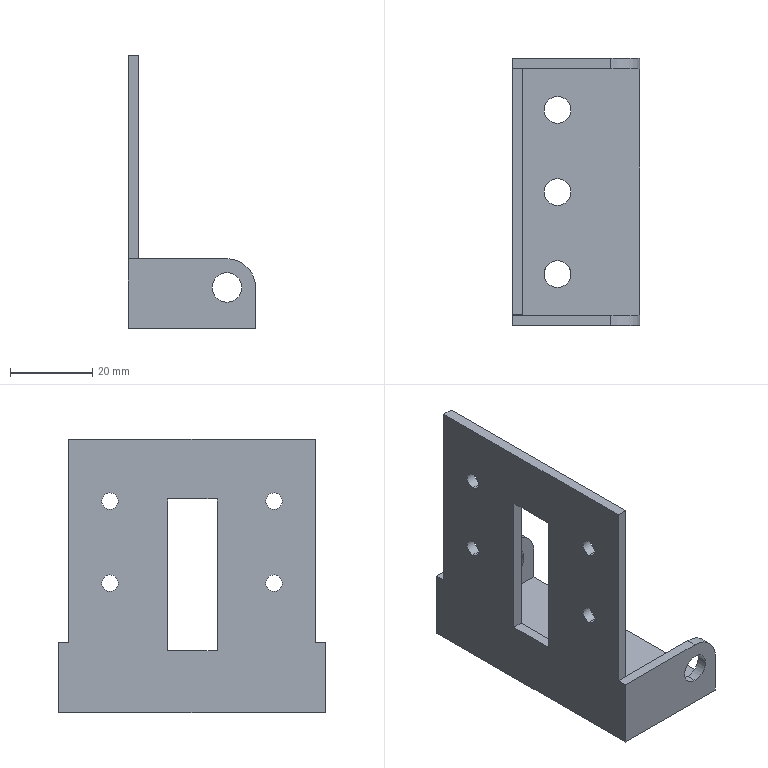Part | SolidWorks | features BaseBody 1 | 1 solid | 38 faces | box 31 x 65 x 66.5 mm | volume 15144 mm3 | cylinder 20 | plane 18 | commonest cylinder face diameters 4 x8 6.5 x6 7.2 x4 14 x2
STEP:
#1=CARTESIAN_POINT('',(875.446,-3880.873,994.471));
#2=VERTEX_POINT('',#1);
#3=CARTESIAN_POINT('',(875.446,-3880.873,998.471));
#4=VERTEX_POINT('',#3);
#5=CARTESIAN_POINT('',(875.446,-3880.873,996.471));
#6=DIRECTION('',(-1.,0.,0.));
#7=DIRECTION('',(0.,0.,1.));
#8=AXIS2_PLACEMENT_3D('',#5,#6,#7);
#9=CIRCLE('',#8,2.);
#10=EDGE_CURVE('',#2,#4,#9,.T.);
#11=ORIENTED_EDGE('',*,*,#10,.F.);
#12=CARTESIAN_POINT('',(872.946,-3880.873,994.471));
#13=VERTEX_POINT('',#12);
#14=CARTESIAN_POINT('',(787.194,-3880.873,994.471));
#15=DIRECTION('',(-1.,0.,0.));
#16=VECTOR('',#15,1000.);
#17=LINE('',#14,#16);
#18=EDGE_CURVE('',#2,#13,#17,.T.);
#19=ORIENTED_EDGE('',*,*,#18,.T.);
#20=CARTESIAN_POINT('',(872.946,-3880.873,998.471));
#21=VERTEX_POINT('',#20);
#22=CARTESIAN_POINT('',(872.946,-3880.873,996.471));
#23=DIRECTION('',(1.,0.,0.));
#24=DIRECTION('',(0.,0.,1.));
#25=AXIS2_PLACEMENT_3D('',#22,#23,#24);
#26=CIRCLE('',#25,2.);
#27=EDGE_CURVE('',#21,#13,#26,.T.);
#28=ORIENTED_EDGE('',*,*,#27,.F.);
#29=CARTESIAN_POINT('',(787.194,-3880.873,998.471));
#30=DIRECTION('',(-1.,0.,0.));
#31=VECTOR('',#30,1000.);
#32=LINE('',#29,#31);
#33=EDGE_CURVE('',#4,#21,#32,.T.);
#34=ORIENTED_EDGE('',*,*,#33,.F.);
#35=EDGE_LOOP('',(#11,#19,#28,#34));
#36=FACE_OUTER_BOUND('',#35,.T.);
#37=CARTESIAN_POINT('',(787.194,-3880.873,996.471));
#38=DIRECTION('',(-1.,0.,0.));
#39=DIRECTION('',(0.,0.,1.));
#40=AXIS2_PLACEMENT_3D('',#37,#38,#39);
#41=CYLINDRICAL_SURFACE('',#40,2.);
#42=ADVANCED_FACE('',(#36),#41,.F.);
#43=CARTESIAN_POINT('',(875.446,-3880.873,974.471));
#44=VERTEX_POINT('',#43);
#45=CARTESIAN_POINT('',(875.446,-3880.873,978.471));
#46=VERTEX_POINT('',#45);
#47=CARTESIAN_POINT('',(875.446,-3880.873,976.471));
#48=DIRECTION('',(-1.,0.,0.));
#49=DIRECTION('',(0.,0.,1.));
#50=AXIS2_PLACEMENT_3D('',#47,#48,#49);
#51=CIRCLE('',#50,2.);
#52=EDGE_CURVE('',#44,#46,#51,.T.);
#53=ORIENTED_EDGE('',*,*,#52,.F.);
#54=CARTESIAN_POINT('',(872.946,-3880.873,974.471));
#55=VERTEX_POINT('',#54);
#56=CARTESIAN_POINT('',(787.194,-3880.873,974.471));
#57=DIRECTION('',(-1.,0.,0.));
#58=VECTOR('',#57,1000.);
#59=LINE('',#56,#58);
#60=EDGE_CURVE('',#44,#55,#59,.T.);
#61=ORIENTED_EDGE('',*,*,#60,.T.);
#62=CARTESIAN_POINT('',(872.946,-3880.873,978.471));
#63=VERTEX_POINT('',#62);
#64=CARTESIAN_POINT('',(872.946,-3880.873,976.471));
#65=DIRECTION('',(1.,0.,0.));
#66=DIRECTION('',(0.,0.,1.));
#67=AXIS2_PLACEMENT_3D('',#64,#65,#66);
#68=CIRCLE('',#67,2.);
#69=EDGE_CURVE('',#63,#55,#68,.T.);
#70=ORIENTED_EDGE('',*,*,#69,.F.);
#71=CARTESIAN_POINT('',(787.194,-3880.873,978.471));
#72=DIRECTION('',(-1.,0.,0.));
#73=VECTOR('',#72,1000.);
#74=LINE('',#71,#73);
#75=EDGE_CURVE('',#46,#63,#74,.T.);
#76=ORIENTED_EDGE('',*,*,#75,.F.);
#77=EDGE_LOOP('',(#53,#61,#70,#76));
#78=FACE_OUTER_BOUND('',#77,.T.);
#79=CARTESIAN_POINT('',(787.194,-3880.873,976.471));
#80=DIRECTION('',(-1.,0.,0.));
#81=DIRECTION('',(0.,0.,1.));
#82=AXIS2_PLACEMENT_3D('',#79,#80,#81);
#83=CYLINDRICAL_SURFACE('',#82,2.);
#84=ADVANCED_FACE('',(#78),#83,.F.);
#85=CARTESIAN_POINT('',(872.946,-3920.873,978.471));
#86=VERTEX_POINT('',#85);
#87=CARTESIAN_POINT('',(872.946,-3920.873,974.471));
#88=VERTEX_POINT('',#87);
#89=CARTESIAN_POINT('',(872.946,-3920.873,976.471));
#90=DIRECTION('',(1.,0.,0.));
#91=DIRECTION('',(0.,0.,-1.));
#92=AXIS2_PLACEMENT_3D('',#89,#90,#91);
#93=CIRCLE('',#92,2.);
#94=EDGE_CURVE('',#86,#88,#93,.T.);
#95=ORIENTED_EDGE('',*,*,#94,.F.);
#96=CARTESIAN_POINT('',(875.446,-3920.873,978.471));
#97=VERTEX_POINT('',#96);
#98=CARTESIAN_POINT('',(787.194,-3920.873,978.471));
#99=DIRECTION('',(1.,0.,0.));
#100=VECTOR('',#99,1000.);
#101=LINE('',#98,#100);
#102=EDGE_CURVE('',#86,#97,#101,.T.);
#103=ORIENTED_EDGE('',*,*,#102,.T.);
#104=CARTESIAN_POINT('',(875.446,-3920.873,974.471));
#105=VERTEX_POINT('',#104);
#106=CARTESIAN_POINT('',(875.446,-3920.873,976.471));
#107=DIRECTION('',(-1.,0.,0.));
#108=DIRECTION('',(0.,0.,-1.));
#109=AXIS2_PLACEMENT_3D('',#106,#107,#108);
#110=CIRCLE('',#109,2.);
#111=EDGE_CURVE('',#105,#97,#110,.T.);
#112=ORIENTED_EDGE('',*,*,#111,.F.);
#113=CARTESIAN_POINT('',(787.194,-3920.873,974.471));
#114=DIRECTION('',(1.,0.,0.));
#115=VECTOR('',#114,1000.);
#116=LINE('',#113,#115);
#117=EDGE_CURVE('',#88,#105,#116,.T.);
#118=ORIENTED_EDGE('',*,*,#117,.F.);
#119=EDGE_LOOP('',(#95,#103,#112,#118));
#120=FACE_OUTER_BOUND('',#119,.T.);
#121=CARTESIAN_POINT('',(787.194,-3920.873,976.471));
#122=DIRECTION('',(1.,0.,0.));
#123=DIRECTION('',(0.,0.,-1.));
#124=AXIS2_PLACEMENT_3D('',#121,#122,#123);
#125=CYLINDRICAL_SURFACE('',#124,2.);
#126=ADVANCED_FACE('',(#120),#125,.F.);
#127=CARTESIAN_POINT('',(872.946,-3920.873,998.471));
#128=VERTEX_POINT('',#127);
#129=CARTESIAN_POINT('',(872.946,-3920.873,994.471));
#130=VERTEX_POINT('',#129);
#131=CARTESIAN_POINT('',(872.946,-3920.873,996.471));
#132=DIRECTION('',(1.,0.,0.));
#133=DIRECTION('',(0.,0.,-1.));
#134=AXIS2_PLACEMENT_3D('',#131,#132,#133);
#135=CIRCLE('',#134,2.);
#136=EDGE_CURVE('',#128,#130,#135,.T.);
#137=ORIENTED_EDGE('',*,*,#136,.F.);
#138=CARTESIAN_POINT('',(875.446,-3920.873,998.471));
#139=VERTEX_POINT('',#138);
#140=CARTESIAN_POINT('',(787.194,-3920.873,998.471));
#141=DIRECTION('',(1.,0.,0.));
#142=VECTOR('',#141,1000.);
#143=LINE('',#140,#142);
#144=EDGE_CURVE('',#128,#139,#143,.T.);
#145=ORIENTED_EDGE('',*,*,#144,.T.);
#146=CARTESIAN_POINT('',(875.446,-3920.873,994.471));
#147=VERTEX_POINT('',#146);
#148=CARTESIAN_POINT('',(875.446,-3920.873,996.471));
#149=DIRECTION('',(-1.,0.,0.));
#150=DIRECTION('',(0.,0.,-1.));
#151=AXIS2_PLACEMENT_3D('',#148,#149,#150);
#152=CIRCLE('',#151,2.);
#153=EDGE_CURVE('',#147,#139,#152,.T.);
#154=ORIENTED_EDGE('',*,*,#153,.F.);
#155=CARTESIAN_POINT('',(787.194,-3920.873,994.471));
#156=DIRECTION('',(1.,0.,0.));
#157=VECTOR('',#156,1000.);
#158=LINE('',#155,#157);
#159=EDGE_CURVE('',#130,#147,#158,.T.);
#160=ORIENTED_EDGE('',*,*,#159,.F.);
#161=EDGE_LOOP('',(#137,#145,#154,#160));
#162=FACE_OUTER_BOUND('',#161,.T.);
#163=CARTESIAN_POINT('',(787.194,-3920.873,996.471));
#164=DIRECTION('',(1.,0.,0.));
#165=DIRECTION('',(0.,0.,-1.));
#166=AXIS2_PLACEMENT_3D('',#163,#164,#165);
#167=CYLINDRICAL_SURFACE('',#166,2.);
#168=ADVANCED_FACE('',(#162),#167,.F.);
#169=CARTESIAN_POINT('',(896.946,-3930.873,958.571));
#170=VERTEX_POINT('',#169);
#171=CARTESIAN_POINT('',(896.946,-3930.873,951.371));
#172=VERTEX_POINT('',#171);
#173=CARTESIAN_POINT('',(896.946,-3930.873,954.971));
#174=DIRECTION('',(0.,-1.,0.));
#175=DIRECTION('',(0.,0.,-1.));
#176=AXIS2_PLACEMENT_3D('',#173,#174,#175);
#177=CIRCLE('',#176,3.6);
#178=EDGE_CURVE('',#170,#172,#177,.T.);
#179=ORIENTED_EDGE('',*,*,#178,.F.);
#180=CARTESIAN_POINT('',(896.946,-3933.373,958.571));
#181=VERTEX_POINT('',#180);
#182=CARTESIAN_POINT('',(896.946,-3930.873,958.571));
#183=DIRECTION('',(0.,-1.,0.));
#184=VECTOR('',#183,1000.);
#185=LINE('',#182,#184);
#186=EDGE_CURVE('',#170,#181,#185,.T.);
#187=ORIENTED_EDGE('',*,*,#186,.T.);
#188=CARTESIAN_POINT('',(896.946,-3933.373,951.371));
#189=VERTEX_POINT('',#188);
#190=CARTESIAN_POINT('',(896.946,-3933.373,954.971));
#191=DIRECTION('',(0.,-1.,0.));
#192=DIRECTION('',(0.,0.,-1.));
#193=AXIS2_PLACEMENT_3D('',#190,#191,#192);
#194=CIRCLE('',#193,3.6);
#195=EDGE_CURVE('',#181,#189,#194,.T.);
#196=ORIENTED_EDGE('',*,*,#195,.T.);
#197=CARTESIAN_POINT('',(896.946,-3930.873,951.371));
#198=DIRECTION('',(0.,-1.,0.));
#199=VECTOR('',#198,1000.);
#200=LINE('',#197,#199);
#201=EDGE_CURVE('',#172,#189,#200,.T.);
#202=ORIENTED_EDGE('',*,*,#201,.F.);
#203=EDGE_LOOP('',(#179,#187,#196,#202));
#204=FACE_OUTER_BOUND('',#203,.T.);
#205=CARTESIAN_POINT('',(896.946,-3930.873,954.971));
#206=DIRECTION('',(0.,-1.,0.));
#207=DIRECTION('',(0.,0.,-1.));
#208=AXIS2_PLACEMENT_3D('',#205,#206,#207);
#209=CYLINDRICAL_SURFACE('',#208,3.6);
#210=ADVANCED_FACE('',(#204),#209,.F.);
#211=CARTESIAN_POINT('',(880.696,-3900.873,944.971));
#212=VERTEX_POINT('',#211);
#213=CARTESIAN_POINT('',(887.196,-3900.873,944.971));
#214=VERTEX_POINT('',#213);
#215=CARTESIAN_POINT('',(883.946,-3900.873,944.971));
#216=DIRECTION('',(0.,0.,1.));
#217=DIRECTION('',(1.,0.,0.));
#218=AXIS2_PLACEMENT_3D('',#215,#216,#217);
#219=CIRCLE('',#218,3.25);
#220=EDGE_CURVE('',#212,#214,#219,.T.);
#221=ORIENTED_EDGE('',*,*,#220,.F.);
#222=CARTESIAN_POINT('',(880.696,-3900.873,947.471));
#223=VERTEX_POINT('',#222);
#224=CARTESIAN_POINT('',(880.696,-3900.873,970.533));
#225=DIRECTION('',(0.,0.,1.));
#226=VECTOR('',#225,1000.);
#227=LINE('',#224,#226);
#228=EDGE_CURVE('',#212,#223,#227,.T.);
#229=ORIENTED_EDGE('',*,*,#228,.T.);
#230=CARTESIAN_POINT('',(887.196,-3900.873,947.471));
#231=VERTEX_POINT('',#230);
#232=CARTESIAN_POINT('',(883.946,-3900.873,947.471));
#233=DIRECTION('',(0.,0.,-1.));
#234=DIRECTION('',(1.,0.,0.));
#235=AXIS2_PLACEMENT_3D('',#232,#233,#234);
#236=CIRCLE('',#235,3.25);
#237=EDGE_CURVE('',#231,#223,#236,.T.);
#238=ORIENTED_EDGE('',*,*,#237,.F.);
#239=CARTESIAN_POINT('',(887.196,-3900.873,970.533));
#240=DIRECTION('',(0.,0.,1.));
#241=VECTOR('',#240,1000.);
#242=LINE('',#239,#241);
#243=EDGE_CURVE('',#214,#231,#242,.T.);
#244=ORIENTED_EDGE('',*,*,#243,.F.);
#245=EDGE_LOOP('',(#221,#229,#238,#244));
#246=FACE_OUTER_BOUND('',#245,.T.);
#247=CARTESIAN_POINT('',(883.946,-3900.873,970.533));
#248=DIRECTION('',(0.,0.,1.));
#249=DIRECTION('',(1.,0.,0.));
#250=AXIS2_PLACEMENT_3D('',#247,#248,#249);
#251=CYLINDRICAL_SURFACE('',#250,3.25);
#252=ADVANCED_FACE('',(#246),#251,.F.);
#253=CARTESIAN_POINT('',(880.696,-3880.873,944.971));
#254=VERTEX_POINT('',#253);
#255=CARTESIAN_POINT('',(887.196,-3880.873,944.971));
#256=VERTEX_POINT('',#255);
#257=CARTESIAN_POINT('',(883.946,-3880.873,944.971));
#258=DIRECTION('',(0.,0.,1.));
#259=DIRECTION('',(1.,0.,0.));
#260=AXIS2_PLACEMENT_3D('',#257,#258,#259);
#261=CIRCLE('',#260,3.25);
#262=EDGE_CURVE('',#254,#256,#261,.T.);
#263=ORIENTED_EDGE('',*,*,#262,.F.);
#264=CARTESIAN_POINT('',(880.696,-3880.873,947.471));
#265=VERTEX_POINT('',#264);
#266=CARTESIAN_POINT('',(880.696,-3880.873,970.533));
#267=DIRECTION('',(0.,0.,1.));
#268=VECTOR('',#267,1000.);
#269=LINE('',#266,#268);
#270=EDGE_CURVE('',#254,#265,#269,.T.);
#271=ORIENTED_EDGE('',*,*,#270,.T.);
#272=CARTESIAN_POINT('',(887.196,-3880.873,947.471));
#273=VERTEX_POINT('',#272);
#274=CARTESIAN_POINT('',(883.946,-3880.873,947.471));
#275=DIRECTION('',(0.,0.,-1.));
#276=DIRECTION('',(1.,0.,0.));
#277=AXIS2_PLACEMENT_3D('',#274,#275,#276);
#278=CIRCLE('',#277,3.25);
#279=EDGE_CURVE('',#273,#265,#278,.T.);
#280=ORIENTED_EDGE('',*,*,#279,.F.);
#281=CARTESIAN_POINT('',(887.196,-3880.873,970.533));
#282=DIRECTION('',(0.,0.,1.));
#283=VECTOR('',#282,1000.);
#284=LINE('',#281,#283);
#285=EDGE_CURVE('',#256,#273,#284,.T.);
#286=ORIENTED_EDGE('',*,*,#285,.F.);
#287=EDGE_LOOP('',(#263,#271,#280,#286));
#288=FACE_OUTER_BOUND('',#287,.T.);
#289=CARTESIAN_POINT('',(883.946,-3880.873,970.533));
#290=DIRECTION('',(0.,0.,1.));
#291=DIRECTION('',(1.,0.,0.));
#292=AXIS2_PLACEMENT_3D('',#289,#290,#291);
#293=CYLINDRICAL_SURFACE('',#292,3.25);
#294=ADVANCED_FACE('',(#288),#293,.F.);
#295=CARTESIAN_POINT('',(880.696,-3920.873,944.971));
#296=VERTEX_POINT('',#295);
#297=CARTESIAN_POINT('',(887.196,-3920.873,944.971));
#298=VERTEX_POINT('',#297);
#299=CARTESIAN_POINT('',(883.946,-3920.873,944.971));
#300=DIRECTION('',(0.,0.,1.));
#301=DIRECTION('',(1.,0.,0.));
#302=AXIS2_PLACEMENT_3D('',#299,#300,#301);
#303=CIRCLE('',#302,3.25);
#304=EDGE_CURVE('',#296,#298,#303,.T.);
#305=ORIENTED_EDGE('',*,*,#304,.F.);
#306=CARTESIAN_POINT('',(880.696,-3920.873,947.471));
#307=VERTEX_POINT('',#306);
#308=CARTESIAN_POINT('',(880.696,-3920.873,970.533));
#309=DIRECTION('',(0.,0.,1.));
#310=VECTOR('',#309,1000.);
#311=LINE('',#308,#310);
#312=EDGE_CURVE('',#296,#307,#311,.T.);
#313=ORIENTED_EDGE('',*,*,#312,.T.);
#314=CARTESIAN_POINT('',(887.196,-3920.873,947.471));
#315=VERTEX_POINT('',#314);
#316=CARTESIAN_POINT('',(883.946,-3920.873,947.471));
#317=DIRECTION('',(0.,0.,-1.));
#318=DIRECTION('',(1.,0.,0.));
#319=AXIS2_PLACEMENT_3D('',#316,#317,#318);
#320=CIRCLE('',#319,3.25);
#321=EDGE_CURVE('',#315,#307,#320,.T.);
#322=ORIENTED_EDGE('',*,*,#321,.F.);
#323=CARTESIAN_POINT('',(887.196,-3920.873,970.533));
#324=DIRECTION('',(0.,0.,1.));
#325=VECTOR('',#324,1000.);
#326=LINE('',#323,#325);
#327=EDGE_CURVE('',#298,#315,#326,.T.);
#328=ORIENTED_EDGE('',*,*,#327,.F.);
#329=EDGE_LOOP('',(#305,#313,#322,#328));
#330=FACE_OUTER_BOUND('',#329,.T.);
#331=CARTESIAN_POINT('',(883.946,-3920.873,970.533));
#332=DIRECTION('',(0.,0.,1.));
#333=DIRECTION('',(1.,0.,0.));
#334=AXIS2_PLACEMENT_3D('',#331,#332,#333);
#335=CYLINDRICAL_SURFACE('',#334,3.25);
#336=ADVANCED_FACE('',(#330),#335,.F.);
#337=CARTESIAN_POINT('',(896.946,-3868.373,951.371));
#338=VERTEX_POINT('',#337);
#339=CARTESIAN_POINT('',(896.946,-3868.373,958.571));
#340=VERTEX_POINT('',#339);
#341=CARTESIAN_POINT('',(896.946,-3868.373,954.971));
#342=DIRECTION('',(0.,1.,0.));
#343=DIRECTION('',(0.,0.,-1.));
#344=AXIS2_PLACEMENT_3D('',#341,#342,#343);
#345=CIRCLE('',#344,3.6);
#346=EDGE_CURVE('',#338,#340,#345,.T.);
#347=ORIENTED_EDGE('',*,*,#346,.T.);
#348=CARTESIAN_POINT('',(896.946,-3870.873,958.571));
#349=VERTEX_POINT('',#348);
#350=CARTESIAN_POINT('',(896.946,-3868.373,958.571));
#351=DIRECTION('',(0.,-1.,0.));
#352=VECTOR('',#351,1000.);
#353=LINE('',#350,#352);
#354=EDGE_CURVE('',#340,#349,#353,.T.);
#355=ORIENTED_EDGE('',*,*,#354,.T.);
#356=CARTESIAN_POINT('',(896.946,-3870.873,951.371));
#357=VERTEX_POINT('',#356);
#358=CARTESIAN_POINT('',(896.946,-3870.873,954.971));
#359=DIRECTION('',(0.,1.,0.));
#360=DIRECTION('',(0.,0.,-1.));
#361=AXIS2_PLACEMENT_3D('',#358,#359,#360);
#362=CIRCLE('',#361,3.6);
#363=EDGE_CURVE('',#357,#349,#362,.T.);
#364=ORIENTED_EDGE('',*,*,#363,.F.);
#365=CARTESIAN_POINT('',(896.946,-3868.373,951.371));
#366=DIRECTION('',(0.,-1.,0.));
#367=VECTOR('',#366,1000.);
#368=LINE('',#365,#367);
#369=EDGE_CURVE('',#338,#357,#368,.T.);
#370=ORIENTED_EDGE('',*,*,#369,.F.);
#371=EDGE_LOOP('',(#347,#355,#364,#370));
#372=FACE_OUTER_BOUND('',#371,.T.);
#373=CARTESIAN_POINT('',(896.946,-3868.373,954.971));
#374=DIRECTION('',(0.,-1.,0.));
#375=DIRECTION('',(0.,0.,-1.));
#376=AXIS2_PLACEMENT_3D('',#373,#374,#375);
#377=CYLINDRICAL_SURFACE('',#376,3.6);
#378=ADVANCED_FACE('',(#372),#377,.F.);
#379=CARTESIAN_POINT('',(872.946,-3870.873,1011.471));
#380=VERTEX_POINT('',#379);
#381=CARTESIAN_POINT('',(872.946,-3870.873,961.971));
#382=VERTEX_POINT('',#381);
#383=CARTESIAN_POINT('',(872.946,-3870.873,951.471));
#384=DIRECTION('',(0.,0.,-1.));
#385=VECTOR('',#384,1000.);
#386=LINE('',#383,#385);
#387=EDGE_CURVE('',#380,#382,#386,.T.);
#388=ORIENTED_EDGE('',*,*,#387,.T.);
#389=CARTESIAN_POINT('',(872.946,-3868.373,961.971));
#390=VERTEX_POINT('',#389);
#391=CARTESIAN_POINT('',(872.946,-3870.873,961.971));
#392=DIRECTION('',(0.,1.,0.));
#393=VECTOR('',#392,1000.);
#394=LINE('',#391,#393);
#395=EDGE_CURVE('',#382,#390,#394,.T.);
#396=ORIENTED_EDGE('',*,*,#395,.T.);
#397=CARTESIAN_POINT('',(872.946,-3868.373,944.971));
#398=VERTEX_POINT('',#397);
#399=CARTESIAN_POINT('',(872.946,-3868.373,951.471));
#400=DIRECTION('',(0.,0.,-1.));
#401=VECTOR('',#400,1000.);
#402=LINE('',#399,#401);
#403=EDGE_CURVE('',#390,#398,#402,.T.);
#404=ORIENTED_EDGE('',*,*,#403,.T.);
#405=CARTESIAN_POINT('',(872.946,-3933.373,944.971));
#406=VERTEX_POINT('',#405);
#407=CARTESIAN_POINT('',(872.946,-3870.873,944.971));
#408=DIRECTION('',(0.,-1.,0.));
#409=VECTOR('',#408,1000.);
#410=LINE('',#407,#409);
#411=EDGE_CURVE('',#398,#406,#410,.T.);
#412=ORIENTED_EDGE('',*,*,#411,.T.);
#413=CARTESIAN_POINT('',(872.946,-3933.373,961.971));
#414=VERTEX_POINT('',#413);
#415=CARTESIAN_POINT('',(872.946,-3933.373,951.471));
#416=DIRECTION('',(0.,0.,1.));
#417=VECTOR('',#416,1000.);
#418=LINE('',#415,#417);
#419=EDGE_CURVE('',#406,#414,#418,.T.);
#420=ORIENTED_EDGE('',*,*,#419,.T.);
#421=CARTESIAN_POINT('',(872.946,-3930.873,961.971));
#422=VERTEX_POINT('',#421);
#423=CARTESIAN_POINT('',(872.946,-3870.873,961.971));
#424=DIRECTION('',(0.,1.,0.));
#425=VECTOR('',#424,1000.);
#426=LINE('',#423,#425);
#427=EDGE_CURVE('',#414,#422,#426,.T.);
#428=ORIENTED_EDGE('',*,*,#427,.T.);
#429=CARTESIAN_POINT('',(872.946,-3930.873,1011.471));
#430=VERTEX_POINT('',#429);
#431=CARTESIAN_POINT('',(872.946,-3930.873,951.471));
#432=DIRECTION('',(0.,0.,1.));
#433=VECTOR('',#432,1000.);
#434=LINE('',#431,#433);
#435=EDGE_CURVE('',#422,#430,#434,.T.);
#436=ORIENTED_EDGE('',*,*,#435,.T.);
#437=CARTESIAN_POINT('',(872.946,-3870.873,1011.471));
#438=DIRECTION('',(0.,1.,0.));
#439=VECTOR('',#438,1000.);
#440=LINE('',#437,#439);
#441=EDGE_CURVE('',#430,#380,#440,.T.);
#442=ORIENTED_EDGE('',*,*,#441,.T.);
#443=EDGE_LOOP('',(#388,#396,#404,#412,#420,#428,#436,#442));
#444=FACE_OUTER_BOUND('',#443,.T.);
#445=CARTESIAN_POINT('',(872.946,-3894.973,959.971));
#446=VERTEX_POINT('',#445);
#447=CARTESIAN_POINT('',(872.946,-3894.973,996.971));
#448=VERTEX_POINT('',#447);
#449=CARTESIAN_POINT('',(872.946,-3894.973,951.471));
#450=DIRECTION('',(0.,0.,1.));
#451=VECTOR('',#450,1000.);
#452=LINE('',#449,#451);
#453=EDGE_CURVE('',#446,#448,#452,.T.);
#454=ORIENTED_EDGE('',*,*,#453,.T.);
#455=CARTESIAN_POINT('',(872.946,-3906.973,996.971));
#456=VERTEX_POINT('',#455);
#457=CARTESIAN_POINT('',(872.946,-3870.873,996.971));
#458=DIRECTION('',(0.,-1.,0.));
#459=VECTOR('',#458,1000.);
#460=LINE('',#457,#459);
#461=EDGE_CURVE('',#448,#456,#460,.T.);
#462=ORIENTED_EDGE('',*,*,#461,.T.);
#463=CARTESIAN_POINT('',(872.946,-3906.973,959.971));
#464=VERTEX_POINT('',#463);
#465=CARTESIAN_POINT('',(872.946,-3906.973,951.471));
#466=DIRECTION('',(0.,0.,-1.));
#467=VECTOR('',#466,1000.);
#468=LINE('',#465,#467);
#469=EDGE_CURVE('',#456,#464,#468,.T.);
#470=ORIENTED_EDGE('',*,*,#469,.T.);
#471=CARTESIAN_POINT('',(872.946,-3870.873,959.971));
#472=DIRECTION('',(0.,1.,0.));
#473=VECTOR('',#472,1000.);
#474=LINE('',#471,#473);
#475=EDGE_CURVE('',#464,#446,#474,.T.);
#476=ORIENTED_EDGE('',*,*,#475,.T.);
#477=EDGE_LOOP('',(#454,#462,#470,#476));
#478=FACE_BOUND('',#477,.T.);
#479=ORIENTED_EDGE('',*,*,#27,.T.);
#480=CARTESIAN_POINT('',(872.946,-3880.873,996.471));
#481=DIRECTION('',(1.,0.,0.));
#482=DIRECTION('',(0.,0.,1.));
#483=AXIS2_PLACEMENT_3D('',#480,#481,#482);
#484=CIRCLE('',#483,2.);
#485=EDGE_CURVE('',#13,#21,#484,.T.);
#486=ORIENTED_EDGE('',*,*,#485,.T.);
#487=EDGE_LOOP('',(#479,#486));
#488=FACE_BOUND('',#487,.T.);
#489=ORIENTED_EDGE('',*,*,#69,.T.);
#490=CARTESIAN_POINT('',(872.946,-3880.873,976.471));
#491=DIRECTION('',(1.,0.,0.));
#492=DIRECTION('',(0.,0.,1.));
#493=AXIS2_PLACEMENT_3D('',#490,#491,#492);
#494=CIRCLE('',#493,2.);
#495=EDGE_CURVE('',#55,#63,#494,.T.);
#496=ORIENTED_EDGE('',*,*,#495,.T.);
#497=EDGE_LOOP('',(#489,#496));
#498=FACE_BOUND('',#497,.T.);
#499=CARTESIAN_POINT('',(872.946,-3920.873,976.471));
#500=DIRECTION('',(1.,0.,0.));
#501=DIRECTION('',(0.,0.,-1.));
#502=AXIS2_PLACEMENT_3D('',#499,#500,#501);
#503=CIRCLE('',#502,2.);
#504=EDGE_CURVE('',#88,#86,#503,.T.);
#505=ORIENTED_EDGE('',*,*,#504,.T.);
#506=ORIENTED_EDGE('',*,*,#94,.T.);
#507=EDGE_LOOP('',(#505,#506));
#508=FACE_BOUND('',#507,.T.);
#509=CARTESIAN_POINT('',(872.946,-3920.873,996.471));
#510=DIRECTION('',(1.,0.,0.));
#511=DIRECTION('',(0.,0.,-1.));
#512=AXIS2_PLACEMENT_3D('',#509,#510,#511);
#513=CIRCLE('',#512,2.);
#514=EDGE_CURVE('',#130,#128,#513,.T.);
#515=ORIENTED_EDGE('',*,*,#514,.T.);
#516=ORIENTED_EDGE('',*,*,#136,.T.);
#517=EDGE_LOOP('',(#515,#516));
#518=FACE_BOUND('',#517,.T.);
#519=CARTESIAN_POINT('',(872.946,-3870.873,951.471));
#520=DIRECTION('',(-1.,0.,0.));
#521=DIRECTION('',(0.,0.,1.));
#522=AXIS2_PLACEMENT_3D('',#519,#520,#521);
#523=PLANE('',#522);
#524=ADVANCED_FACE('',(#444,#478,#488,#498,#508,#518),#523,.T.);
#525=CARTESIAN_POINT('',(875.446,-3870.873,961.971));
#526=VERTEX_POINT('',#525);
#527=CARTESIAN_POINT('',(896.946,-3870.873,961.971));
#528=VERTEX_POINT('',#527);
#529=CARTESIAN_POINT('',(872.946,-3870.873,961.971));
#530=DIRECTION('',(1.,0.,0.));
#531=VECTOR('',#530,1000.);
#532=LINE('',#529,#531);
#533=EDGE_CURVE('',#526,#528,#532,.T.);
#534=ORIENTED_EDGE('',*,*,#533,.T.);
#535=CARTESIAN_POINT('',(896.946,-3868.373,961.971));
#536=VERTEX_POINT('',#535);
#537=CARTESIAN_POINT('',(896.946,-3870.873,961.971));
#538=DIRECTION('',(0.,1.,0.));
#539=VECTOR('',#538,1000.);
#540=LINE('',#537,#539);
#541=EDGE_CURVE('',#528,#536,#540,.T.);
#542=ORIENTED_EDGE('',*,*,#541,.T.);
#543=CARTESIAN_POINT('',(872.946,-3868.373,961.971));
#544=DIRECTION('',(-1.,0.,0.));
#545=VECTOR('',#544,1000.);
#546=LINE('',#543,#545);
#547=EDGE_CURVE('',#536,#390,#546,.T.);
#548=ORIENTED_EDGE('',*,*,#547,.T.);
#549=ORIENTED_EDGE('',*,*,#395,.F.);
#550=CARTESIAN_POINT('',(872.946,-3870.873,961.971));
#551=DIRECTION('',(1.,0.,0.));
#552=VECTOR('',#551,1000.);
#553=LINE('',#550,#552);
#554=EDGE_CURVE('',#382,#526,#553,.T.);
#555=ORIENTED_EDGE('',*,*,#554,.T.);
#556=EDGE_LOOP('',(#534,#542,#548,#549,#555));
#557=FACE_OUTER_BOUND('',#556,.T.);
#558=CARTESIAN_POINT('',(872.946,-3870.873,961.971));
#559=DIRECTION('',(0.,0.,1.));
#560=DIRECTION('',(1.,0.,0.));
#561=AXIS2_PLACEMENT_3D('',#558,#559,#560);
#562=PLANE('',#561);
#563=ADVANCED_FACE('',(#557),#562,.T.);
#564=CARTESIAN_POINT('',(875.446,-3870.873,1011.471));
#565=VERTEX_POINT('',#564);
#566=CARTESIAN_POINT('',(879.441,-3870.873,1011.471));
#567=DIRECTION('',(1.,0.,0.));
#568=VECTOR('',#567,1000.);
#569=LINE('',#566,#568);
#570=EDGE_CURVE('',#380,#565,#569,.T.);
#571=ORIENTED_EDGE('',*,*,#570,.T.);
#572=CARTESIAN_POINT('',(875.446,-3870.873,965.967));
#573=DIRECTION('',(0.,0.,-1.));
#574=VECTOR('',#573,1000.);
#575=LINE('',#572,#574);
#576=EDGE_CURVE('',#565,#526,#575,.T.);
#577=ORIENTED_EDGE('',*,*,#576,.T.);
#578=ORIENTED_EDGE('',*,*,#554,.F.);
#579=ORIENTED_EDGE('',*,*,#387,.F.);
#580=EDGE_LOOP('',(#571,#577,#578,#579));
#581=FACE_OUTER_BOUND('',#580,.T.);
#582=CARTESIAN_POINT('',(879.441,-3870.873,965.967));
#583=DIRECTION('',(0.,1.,0.));
#584=DIRECTION('',(0.,0.,1.));
#585=AXIS2_PLACEMENT_3D('',#582,#583,#584);
#586=PLANE('',#585);
#587=ADVANCED_FACE('',(#581),#586,.T.);
#588=ORIENTED_EDGE('',*,*,#570,.F.);
#589=ORIENTED_EDGE('',*,*,#441,.F.);
#590=CARTESIAN_POINT('',(875.446,-3930.873,1011.471));
#591=VERTEX_POINT('',#590);
#592=CARTESIAN_POINT('',(872.946,-3930.873,1011.471));
#593=DIRECTION('',(1.,0.,0.));
#594=VECTOR('',#593,1000.);
#595=LINE('',#592,#594);
#596=EDGE_CURVE('',#430,#591,#595,.T.);
#597=ORIENTED_EDGE('',*,*,#596,.T.);
#598=CARTESIAN_POINT('',(875.446,-3870.873,1011.471));
#599=DIRECTION('',(0.,1.,0.));
#600=VECTOR('',#599,1000.);
#601=LINE('',#598,#600);
#602=EDGE_CURVE('',#591,#565,#601,.T.);
#603=ORIENTED_EDGE('',*,*,#602,.T.);
#604=EDGE_LOOP('',(#588,#589,#597,#603));
#605=FACE_OUTER_BOUND('',#604,.T.);
#606=CARTESIAN_POINT('',(872.946,-3870.873,1011.471));
#607=DIRECTION('',(0.,0.,1.));
#608=DIRECTION('',(1.,0.,0.));
#609=AXIS2_PLACEMENT_3D('',#606,#607,#608);
#610=PLANE('',#609);
#611=ADVANCED_FACE('',(#605),#610,.T.);
#612=CARTESIAN_POINT('',(875.446,-3930.873,961.971));
#613=VERTEX_POINT('',#612);
#614=CARTESIAN_POINT('',(875.446,-3930.873,965.967));
#615=DIRECTION('',(0.,0.,-1.));
#616=VECTOR('',#615,1000.);
#617=LINE('',#614,#616);
#618=EDGE_CURVE('',#591,#613,#617,.T.);
#619=ORIENTED_EDGE('',*,*,#618,.F.);
#620=ORIENTED_EDGE('',*,*,#596,.F.);
#621=ORIENTED_EDGE('',*,*,#435,.F.);
#622=CARTESIAN_POINT('',(879.441,-3930.873,961.971));
#623=DIRECTION('',(-1.,0.,0.));
#624=VECTOR('',#623,1000.);
#625=LINE('',#622,#624);
#626=EDGE_CURVE('',#613,#422,#625,.T.);
#627=ORIENTED_EDGE('',*,*,#626,.F.);
#628=EDGE_LOOP('',(#619,#620,#621,#627));
#629=FACE_OUTER_BOUND('',#628,.T.);
#630=CARTESIAN_POINT('',(879.441,-3930.873,965.967));
#631=DIRECTION('',(0.,1.,0.));
#632=DIRECTION('',(0.,0.,1.));
#633=AXIS2_PLACEMENT_3D('',#630,#631,#632);
#634=PLANE('',#633);
#635=ADVANCED_FACE('',(#629),#634,.F.);
#636=ORIENTED_EDGE('',*,*,#626,.T.);
#637=ORIENTED_EDGE('',*,*,#427,.F.);
#638=CARTESIAN_POINT('',(896.946,-3933.373,961.971));
#639=VERTEX_POINT('',#638);
#640=CARTESIAN_POINT('',(872.946,-3933.373,961.971));
#641=DIRECTION('',(1.,0.,0.));
#642=VECTOR('',#641,1000.);
#643=LINE('',#640,#642);
#644=EDGE_CURVE('',#414,#639,#643,.T.);
#645=ORIENTED_EDGE('',*,*,#644,.T.);
#646=CARTESIAN_POINT('',(896.946,-3930.873,961.971));
#647=VERTEX_POINT('',#646);
#648=CARTESIAN_POINT('',(896.946,-3930.873,961.971));
#649=DIRECTION('',(0.,1.,0.));
#650=VECTOR('',#649,1000.);
#651=LINE('',#648,#650);
#652=EDGE_CURVE('',#639,#647,#651,.T.);
#653=ORIENTED_EDGE('',*,*,#652,.T.);
#654=CARTESIAN_POINT('',(872.946,-3930.873,961.971));
#655=DIRECTION('',(-1.,0.,0.));
#656=VECTOR('',#655,1000.);
#657=LINE('',#654,#656);
#658=EDGE_CURVE('',#647,#613,#657,.T.);
#659=ORIENTED_EDGE('',*,*,#658,.T.);
#660=EDGE_LOOP('',(#636,#637,#645,#653,#659));
#661=FACE_OUTER_BOUND('',#660,.T.);
#662=CARTESIAN_POINT('',(872.946,-3930.873,961.971));
#663=DIRECTION('',(0.,0.,1.));
#664=DIRECTION('',(1.,0.,0.));
#665=AXIS2_PLACEMENT_3D('',#662,#663,#664);
#666=PLANE('',#665);
#667=ADVANCED_FACE('',(#661),#666,.T.);
#668=CARTESIAN_POINT('',(903.946,-3933.373,954.971));
#669=VERTEX_POINT('',#668);
#670=CARTESIAN_POINT('',(903.946,-3933.373,944.971));
#671=VERTEX_POINT('',#670);
#672=CARTESIAN_POINT('',(903.946,-3933.373,953.148));
#673=DIRECTION('',(0.,0.,-1.));
#674=VECTOR('',#673,1000.);
#675=LINE('',#672,#674);
#676=EDGE_CURVE('',#669,#671,#675,.T.);
#677=ORIENTED_EDGE('',*,*,#676,.F.);
#678=CARTESIAN_POINT('',(896.946,-3933.373,954.971));
#679=DIRECTION('',(0.,1.,0.));
#680=DIRECTION('',(0.,0.,-1.));
#681=AXIS2_PLACEMENT_3D('',#678,#679,#680);
#682=CIRCLE('',#681,7.);
#683=EDGE_CURVE('',#639,#669,#682,.T.);
#684=ORIENTED_EDGE('',*,*,#683,.F.);
#685=ORIENTED_EDGE('',*,*,#644,.F.);
#686=ORIENTED_EDGE('',*,*,#419,.F.);
#687=CARTESIAN_POINT('',(887.896,-3933.373,944.971));
#688=DIRECTION('',(-1.,0.,0.));
#689=VECTOR('',#688,1000.);
#690=LINE('',#687,#689);
#691=EDGE_CURVE('',#671,#406,#690,.T.);
#692=ORIENTED_EDGE('',*,*,#691,.F.);
#693=EDGE_LOOP('',(#677,#684,#685,#686,#692));
#694=FACE_OUTER_BOUND('',#693,.T.);
#695=CARTESIAN_POINT('',(896.946,-3933.373,954.971));
#696=DIRECTION('',(0.,-1.,0.));
#697=DIRECTION('',(0.,0.,-1.));
#698=AXIS2_PLACEMENT_3D('',#695,#696,#697);
#699=CIRCLE('',#698,3.6);
#700=EDGE_CURVE('',#189,#181,#699,.T.);
#701=ORIENTED_EDGE('',*,*,#700,.F.);
#702=ORIENTED_EDGE('',*,*,#195,.F.);
#703=EDGE_LOOP('',(#701,#702));
#704=FACE_BOUND('',#703,.T.);
#705=CARTESIAN_POINT('',(887.896,-3933.373,953.148));
#706=DIRECTION('',(0.,1.,0.));
#707=DIRECTION('',(0.,0.,1.));
#708=AXIS2_PLACEMENT_3D('',#705,#706,#707);
#709=PLANE('',#708);
#710=ADVANCED_FACE('',(#694,#704),#709,.F.);
#711=ORIENTED_EDGE('',*,*,#691,.T.);
#712=ORIENTED_EDGE('',*,*,#411,.F.);
#713=CARTESIAN_POINT('',(903.946,-3868.373,944.971));
#714=VERTEX_POINT('',#713);
#715=CARTESIAN_POINT('',(903.946,-3868.373,944.971));
#716=DIRECTION('',(1.,0.,0.));
#717=VECTOR('',#716,1000.);
#718=LINE('',#715,#717);
#719=EDGE_CURVE('',#398,#714,#718,.T.);
#720=ORIENTED_EDGE('',*,*,#719,.T.);
#721=CARTESIAN_POINT('',(903.946,-3870.873,944.971));
#722=DIRECTION('',(0.,-1.,0.));
#723=VECTOR('',#722,1000.);
#724=LINE('',#721,#723);
#725=EDGE_CURVE('',#714,#671,#724,.T.);
#726=ORIENTED_EDGE('',*,*,#725,.T.);
#727=EDGE_LOOP('',(#711,#712,#720,#726));
#728=FACE_OUTER_BOUND('',#727,.T.);
#729=CARTESIAN_POINT('',(883.946,-3900.873,944.971));
#730=DIRECTION('',(0.,0.,1.));
#731=DIRECTION('',(1.,0.,0.));
#732=AXIS2_PLACEMENT_3D('',#729,#730,#731);
#733=CIRCLE('',#732,3.25);
#734=EDGE_CURVE('',#214,#212,#733,.T.);
#735=ORIENTED_EDGE('',*,*,#734,.T.);
#736=ORIENTED_EDGE('',*,*,#220,.T.);
#737=EDGE_LOOP('',(#735,#736));
#738=FACE_BOUND('',#737,.T.);
#739=CARTESIAN_POINT('',(883.946,-3880.873,944.971));
#740=DIRECTION('',(0.,0.,1.));
#741=DIRECTION('',(1.,0.,0.));
#742=AXIS2_PLACEMENT_3D('',#739,#740,#741);
#743=CIRCLE('',#742,3.25);
#744=EDGE_CURVE('',#256,#254,#743,.T.);
#745=ORIENTED_EDGE('',*,*,#744,.T.);
#746=ORIENTED_EDGE('',*,*,#262,.T.);
#747=EDGE_LOOP('',(#745,#746));
#748=FACE_BOUND('',#747,.T.);
#749=CARTESIAN_POINT('',(883.946,-3920.873,944.971));
#750=DIRECTION('',(0.,0.,1.));
#751=DIRECTION('',(1.,0.,0.));
#752=AXIS2_PLACEMENT_3D('',#749,#750,#751);
#753=CIRCLE('',#752,3.25);
#754=EDGE_CURVE('',#298,#296,#753,.T.);
#755=ORIENTED_EDGE('',*,*,#754,.T.);
#756=ORIENTED_EDGE('',*,*,#304,.T.);
#757=EDGE_LOOP('',(#755,#756));
#758=FACE_BOUND('',#757,.T.);
#759=CARTESIAN_POINT('',(903.946,-3870.873,944.971));
#760=DIRECTION('',(0.,0.,-1.));
#761=DIRECTION('',(-1.,0.,0.));
#762=AXIS2_PLACEMENT_3D('',#759,#760,#761);
#763=PLANE('',#762);
#764=ADVANCED_FACE('',(#728,#738,#748,#758),#763,.T.);
#765=ORIENTED_EDGE('',*,*,#403,.F.);
#766=ORIENTED_EDGE('',*,*,#547,.F.);
#767=CARTESIAN_POINT('',(903.946,-3868.373,954.971));
#768=VERTEX_POINT('',#767);
#769=CARTESIAN_POINT('',(896.946,-3868.373,954.971));
#770=DIRECTION('',(0.,-1.,0.));
#771=DIRECTION('',(0.,0.,-1.));
#772=AXIS2_PLACEMENT_3D('',#769,#770,#771);
#773=CIRCLE('',#772,7.);
#774=EDGE_CURVE('',#768,#536,#773,.T.);
#775=ORIENTED_EDGE('',*,*,#774,.F.);
#776=CARTESIAN_POINT('',(903.946,-3868.373,953.148));
#777=DIRECTION('',(0.,0.,1.));
#778=VECTOR('',#777,1000.);
#779=LINE('',#776,#778);
#780=EDGE_CURVE('',#714,#768,#779,.T.);
#781=ORIENTED_EDGE('',*,*,#780,.F.);
#782=ORIENTED_EDGE('',*,*,#719,.F.);
#783=EDGE_LOOP('',(#765,#766,#775,#781,#782));
#784=FACE_OUTER_BOUND('',#783,.T.);
#785=ORIENTED_EDGE('',*,*,#346,.F.);
#786=CARTESIAN_POINT('',(896.946,-3868.373,954.971));
#787=DIRECTION('',(0.,1.,0.));
#788=DIRECTION('',(0.,0.,-1.));
#789=AXIS2_PLACEMENT_3D('',#786,#787,#788);
#790=CIRCLE('',#789,3.6);
#791=EDGE_CURVE('',#340,#338,#790,.T.);
#792=ORIENTED_EDGE('',*,*,#791,.F.);
#793=EDGE_LOOP('',(#785,#792));
#794=FACE_BOUND('',#793,.T.);
#795=CARTESIAN_POINT('',(887.896,-3868.373,953.148));
#796=DIRECTION('',(0.,-1.,0.));
#797=DIRECTION('',(0.,0.,-1.));
#798=AXIS2_PLACEMENT_3D('',#795,#796,#797);
#799=PLANE('',#798);
#800=ADVANCED_FACE('',(#784,#794),#799,.F.);
#801=CARTESIAN_POINT('',(875.446,-3906.973,996.971));
#802=VERTEX_POINT('',#801);
#803=CARTESIAN_POINT('',(884.977,-3906.973,996.971));
#804=DIRECTION('',(1.,0.,0.));
#805=VECTOR('',#804,1000.);
#806=LINE('',#803,#805);
#807=EDGE_CURVE('',#456,#802,#806,.T.);
#808=ORIENTED_EDGE('',*,*,#807,.F.);
#809=ORIENTED_EDGE('',*,*,#461,.F.);
#810=CARTESIAN_POINT('',(875.446,-3894.973,996.971));
#811=VERTEX_POINT('',#810);
#812=CARTESIAN_POINT('',(884.977,-3894.973,996.971));
#813=DIRECTION('',(-1.,0.,0.));
#814=VECTOR('',#813,1000.);
#815=LINE('',#812,#814);
#816=EDGE_CURVE('',#811,#448,#815,.T.);
#817=ORIENTED_EDGE('',*,*,#816,.F.);
#818=CARTESIAN_POINT('',(875.446,-3894.973,996.971));
#819=DIRECTION('',(0.,1.,0.));
#820=VECTOR('',#819,1000.);
#821=LINE('',#818,#820);
#822=EDGE_CURVE('',#802,#811,#821,.T.);
#823=ORIENTED_EDGE('',*,*,#822,.F.);
#824=EDGE_LOOP('',(#808,#809,#817,#823));
#825=FACE_OUTER_BOUND('',#824,.T.);
#826=CARTESIAN_POINT('',(884.977,-3894.973,996.971));
#827=DIRECTION('',(0.,0.,1.));
#828=DIRECTION('',(1.,0.,0.));
#829=AXIS2_PLACEMENT_3D('',#826,#827,#828);
#830=PLANE('',#829);
#831=ADVANCED_FACE('',(#825),#830,.F.);
#832=ORIENTED_EDGE('',*,*,#816,.T.);
#833=ORIENTED_EDGE('',*,*,#453,.F.);
#834=CARTESIAN_POINT('',(875.446,-3894.973,959.971));
#835=VERTEX_POINT('',#834);
#836=CARTESIAN_POINT('',(884.977,-3894.973,959.971));
#837=DIRECTION('',(-1.,0.,0.));
#838=VECTOR('',#837,1000.);
#839=LINE('',#836,#838);
#840=EDGE_CURVE('',#835,#446,#839,.T.);
#841=ORIENTED_EDGE('',*,*,#840,.F.);
#842=CARTESIAN_POINT('',(875.446,-3894.973,959.971));
#843=DIRECTION('',(0.,0.,-1.));
#844=VECTOR('',#843,1000.);
#845=LINE('',#842,#844);
#846=EDGE_CURVE('',#811,#835,#845,.T.);
#847=ORIENTED_EDGE('',*,*,#846,.F.);
#848=EDGE_LOOP('',(#832,#833,#841,#847));
#849=FACE_OUTER_BOUND('',#848,.T.);
#850=CARTESIAN_POINT('',(884.977,-3894.973,959.971));
#851=DIRECTION('',(0.,1.,0.));
#852=DIRECTION('',(0.,0.,1.));
#853=AXIS2_PLACEMENT_3D('',#850,#851,#852);
#854=PLANE('',#853);
#855=ADVANCED_FACE('',(#849),#854,.F.);
#856=ORIENTED_EDGE('',*,*,#840,.T.);
#857=ORIENTED_EDGE('',*,*,#475,.F.);
#858=CARTESIAN_POINT('',(875.446,-3906.973,959.971));
#859=VERTEX_POINT('',#858);
#860=CARTESIAN_POINT('',(884.977,-3906.973,959.971));
#861=DIRECTION('',(-1.,0.,0.));
#862=VECTOR('',#861,1000.);
#863=LINE('',#860,#862);
#864=EDGE_CURVE('',#859,#464,#863,.T.);
#865=ORIENTED_EDGE('',*,*,#864,.F.);
#866=CARTESIAN_POINT('',(875.446,-3906.973,959.971));
#867=DIRECTION('',(0.,-1.,0.));
#868=VECTOR('',#867,1000.);
#869=LINE('',#866,#868);
#870=EDGE_CURVE('',#835,#859,#869,.T.);
#871=ORIENTED_EDGE('',*,*,#870,.F.);
#872=EDGE_LOOP('',(#856,#857,#865,#871));
#873=FACE_OUTER_BOUND('',#872,.T.);
#874=CARTESIAN_POINT('',(884.977,-3906.973,959.971));
#875=DIRECTION('',(0.,0.,-1.));
#876=DIRECTION('',(-1.,0.,0.));
#877=AXIS2_PLACEMENT_3D('',#874,#875,#876);
#878=PLANE('',#877);
#879=ADVANCED_FACE('',(#873),#878,.F.);
#880=ORIENTED_EDGE('',*,*,#864,.T.);
#881=ORIENTED_EDGE('',*,*,#469,.F.);
#882=ORIENTED_EDGE('',*,*,#807,.T.);
#883=CARTESIAN_POINT('',(875.446,-3906.973,996.971));
#884=DIRECTION('',(0.,0.,1.));
#885=VECTOR('',#884,1000.);
#886=LINE('',#883,#885);
#887=EDGE_CURVE('',#859,#802,#886,.T.);
#888=ORIENTED_EDGE('',*,*,#887,.F.);
#889=EDGE_LOOP('',(#880,#881,#882,#888));
#890=FACE_OUTER_BOUND('',#889,.T.);
#891=CARTESIAN_POINT('',(884.977,-3906.973,996.971));
#892=DIRECTION('',(0.,-1.,0.));
#893=DIRECTION('',(0.,0.,-1.));
#894=AXIS2_PLACEMENT_3D('',#891,#892,#893);
#895=PLANE('',#894);
#896=ADVANCED_FACE('',(#890),#895,.F.);
#897=ORIENTED_EDGE('',*,*,#18,.F.);
#898=CARTESIAN_POINT('',(875.446,-3880.873,996.471));
#899=DIRECTION('',(-1.,0.,0.));
#900=DIRECTION('',(0.,0.,1.));
#901=AXIS2_PLACEMENT_3D('',#898,#899,#900);
#902=CIRCLE('',#901,2.);
#903=EDGE_CURVE('',#4,#2,#902,.T.);
#904=ORIENTED_EDGE('',*,*,#903,.F.);
#905=ORIENTED_EDGE('',*,*,#33,.T.);
#906=ORIENTED_EDGE('',*,*,#485,.F.);
#907=EDGE_LOOP('',(#897,#904,#905,#906));
#908=FACE_OUTER_BOUND('',#907,.T.);
#909=CARTESIAN_POINT('',(787.194,-3880.873,996.471));
#910=DIRECTION('',(-1.,0.,0.));
#911=DIRECTION('',(0.,0.,1.));
#912=AXIS2_PLACEMENT_3D('',#909,#910,#911);
#913=CYLINDRICAL_SURFACE('',#912,2.);
#914=ADVANCED_FACE('',(#908),#913,.F.);
#915=ORIENTED_EDGE('',*,*,#60,.F.);
#916=CARTESIAN_POINT('',(875.446,-3880.873,976.471));
#917=DIRECTION('',(-1.,0.,0.));
#918=DIRECTION('',(0.,0.,1.));
#919=AXIS2_PLACEMENT_3D('',#916,#917,#918);
#920=CIRCLE('',#919,2.);
#921=EDGE_CURVE('',#46,#44,#920,.T.);
#922=ORIENTED_EDGE('',*,*,#921,.F.);
#923=ORIENTED_EDGE('',*,*,#75,.T.);
#924=ORIENTED_EDGE('',*,*,#495,.F.);
#925=EDGE_LOOP('',(#915,#922,#923,#924));
#926=FACE_OUTER_BOUND('',#925,.T.);
#927=CARTESIAN_POINT('',(787.194,-3880.873,976.471));
#928=DIRECTION('',(-1.,0.,0.));
#929=DIRECTION('',(0.,0.,1.));
#930=AXIS2_PLACEMENT_3D('',#927,#928,#929);
#931=CYLINDRICAL_SURFACE('',#930,2.);
#932=ADVANCED_FACE('',(#926),#931,.F.);
#933=ORIENTED_EDGE('',*,*,#102,.F.);
#934=ORIENTED_EDGE('',*,*,#504,.F.);
#935=ORIENTED_EDGE('',*,*,#117,.T.);
#936=CARTESIAN_POINT('',(875.446,-3920.873,976.471));
#937=DIRECTION('',(-1.,0.,0.));
#938=DIRECTION('',(0.,0.,-1.));
#939=AXIS2_PLACEMENT_3D('',#936,#937,#938);
#940=CIRCLE('',#939,2.);
#941=EDGE_CURVE('',#97,#105,#940,.T.);
#942=ORIENTED_EDGE('',*,*,#941,.F.);
#943=EDGE_LOOP('',(#933,#934,#935,#942));
#944=FACE_OUTER_BOUND('',#943,.T.);
#945=CARTESIAN_POINT('',(787.194,-3920.873,976.471));
#946=DIRECTION('',(1.,0.,0.));
#947=DIRECTION('',(0.,0.,-1.));
#948=AXIS2_PLACEMENT_3D('',#945,#946,#947);
#949=CYLINDRICAL_SURFACE('',#948,2.);
#950=ADVANCED_FACE('',(#944),#949,.F.);
#951=ORIENTED_EDGE('',*,*,#144,.F.);
#952=ORIENTED_EDGE('',*,*,#514,.F.);
#953=ORIENTED_EDGE('',*,*,#159,.T.);
#954=CARTESIAN_POINT('',(875.446,-3920.873,996.471));
#955=DIRECTION('',(-1.,0.,0.));
#956=DIRECTION('',(0.,0.,-1.));
#957=AXIS2_PLACEMENT_3D('',#954,#955,#956);
#958=CIRCLE('',#957,2.);
#959=EDGE_CURVE('',#139,#147,#958,.T.);
#960=ORIENTED_EDGE('',*,*,#959,.F.);
#961=EDGE_LOOP('',(#951,#952,#953,#960));
#962=FACE_OUTER_BOUND('',#961,.T.);
#963=CARTESIAN_POINT('',(787.194,-3920.873,996.471));
#964=DIRECTION('',(1.,0.,0.));
#965=DIRECTION('',(0.,0.,-1.));
#966=AXIS2_PLACEMENT_3D('',#963,#964,#965);
#967=CYLINDRICAL_SURFACE('',#966,2.);
#968=ADVANCED_FACE('',(#962),#967,.F.);
#969=CARTESIAN_POINT('',(903.946,-3870.873,954.971));
#970=VERTEX_POINT('',#969);
#971=CARTESIAN_POINT('',(896.946,-3870.873,954.971));
#972=DIRECTION('',(0.,1.,0.));
#973=DIRECTION('',(0.,0.,-1.));
#974=AXIS2_PLACEMENT_3D('',#971,#972,#973);
#975=CIRCLE('',#974,7.);
#976=EDGE_CURVE('',#528,#970,#975,.T.);
#977=ORIENTED_EDGE('',*,*,#976,.T.);
#978=CARTESIAN_POINT('',(903.946,-3870.873,954.971));
#979=DIRECTION('',(0.,1.,0.));
#980=VECTOR('',#979,1000.);
#981=LINE('',#978,#980);
#982=EDGE_CURVE('',#970,#768,#981,.T.);
#983=ORIENTED_EDGE('',*,*,#982,.T.);
#984=ORIENTED_EDGE('',*,*,#774,.T.);
#985=ORIENTED_EDGE('',*,*,#541,.F.);
#986=EDGE_LOOP('',(#977,#983,#984,#985));
#987=FACE_OUTER_BOUND('',#986,.T.);
#988=CARTESIAN_POINT('',(896.946,-3870.873,954.971));
#989=DIRECTION('',(0.,-1.,0.));
#990=DIRECTION('',(0.,0.,-1.));
#991=AXIS2_PLACEMENT_3D('',#988,#989,#990);
#992=CYLINDRICAL_SURFACE('',#991,7.);
#993=ADVANCED_FACE('',(#987),#992,.T.);
#994=ORIENTED_EDGE('',*,*,#363,.T.);
#995=CARTESIAN_POINT('',(896.946,-3870.873,954.971));
#996=DIRECTION('',(0.,1.,0.));
#997=DIRECTION('',(0.,0.,-1.));
#998=AXIS2_PLACEMENT_3D('',#995,#996,#997);
#999=CIRCLE('',#998,3.6);
#1000=EDGE_CURVE('',#349,#357,#999,.T.);
#1001=ORIENTED_EDGE('',*,*,#1000,.T.);
#1002=EDGE_LOOP('',(#994,#1001));
#1003=FACE_BOUND('',#1002,.T.);
#1004=ORIENTED_EDGE('',*,*,#533,.F.);
#1005=CARTESIAN_POINT('',(875.446,-3870.873,947.471));
#1006=VERTEX_POINT('',#1005);
#1007=CARTESIAN_POINT('',(875.446,-3870.873,953.148));
#1008=DIRECTION('',(0.,0.,-1.));
#1009=VECTOR('',#1008,1000.);
#1010=LINE('',#1007,#1009);
#1011=EDGE_CURVE('',#526,#1006,#1010,.T.);
#1012=ORIENTED_EDGE('',*,*,#1011,.T.);
#1013=CARTESIAN_POINT('',(903.946,-3870.873,947.471));
#1014=VERTEX_POINT('',#1013);
#1015=CARTESIAN_POINT('',(887.896,-3870.873,947.471));
#1016=DIRECTION('',(1.,0.,0.));
#1017=VECTOR('',#1016,1000.);
#1018=LINE('',#1015,#1017);
#1019=EDGE_CURVE('',#1006,#1014,#1018,.T.);
#1020=ORIENTED_EDGE('',*,*,#1019,.T.);
#1021=CARTESIAN_POINT('',(903.946,-3870.873,953.148));
#1022=DIRECTION('',(0.,0.,1.));
#1023=VECTOR('',#1022,1000.);
#1024=LINE('',#1021,#1023);
#1025=EDGE_CURVE('',#1014,#970,#1024,.T.);
#1026=ORIENTED_EDGE('',*,*,#1025,.T.);
#1027=ORIENTED_EDGE('',*,*,#976,.F.);
#1028=EDGE_LOOP('',(#1004,#1012,#1020,#1026,#1027));
#1029=FACE_OUTER_BOUND('',#1028,.T.);
#1030=CARTESIAN_POINT('',(887.896,-3870.873,953.148));
#1031=DIRECTION('',(0.,-1.,0.));
#1032=DIRECTION('',(0.,0.,-1.));
#1033=AXIS2_PLACEMENT_3D('',#1030,#1031,#1032);
#1034=PLANE('',#1033);
#1035=ADVANCED_FACE('',(#1003,#1029),#1034,.T.);
#1036=ORIENTED_EDGE('',*,*,#576,.F.);
#1037=ORIENTED_EDGE('',*,*,#602,.F.);
#1038=ORIENTED_EDGE('',*,*,#618,.T.);
#1039=CARTESIAN_POINT('',(875.446,-3930.873,947.471));
#1040=VERTEX_POINT('',#1039);
#1041=CARTESIAN_POINT('',(875.446,-3930.873,1004.971));
#1042=DIRECTION('',(0.,0.,-1.));
#1043=VECTOR('',#1042,1000.);
#1044=LINE('',#1041,#1043);
#1045=EDGE_CURVE('',#613,#1040,#1044,.T.);
#1046=ORIENTED_EDGE('',*,*,#1045,.T.);
#1047=CARTESIAN_POINT('',(875.446,-3870.873,947.471));
#1048=DIRECTION('',(0.,1.,0.));
#1049=VECTOR('',#1048,1000.);
#1050=LINE('',#1047,#1049);
#1051=EDGE_CURVE('',#1040,#1006,#1050,.T.);
#1052=ORIENTED_EDGE('',*,*,#1051,.T.);
#1053=ORIENTED_EDGE('',*,*,#1011,.F.);
#1054=EDGE_LOOP('',(#1036,#1037,#1038,#1046,#1052,#1053));
#1055=FACE_OUTER_BOUND('',#1054,.T.);
#1056=ORIENTED_EDGE('',*,*,#846,.T.);
#1057=ORIENTED_EDGE('',*,*,#870,.T.);
#1058=ORIENTED_EDGE('',*,*,#887,.T.);
#1059=ORIENTED_EDGE('',*,*,#822,.T.);
#1060=EDGE_LOOP('',(#1056,#1057,#1058,#1059));
#1061=FACE_BOUND('',#1060,.T.);
#1062=ORIENTED_EDGE('',*,*,#903,.T.);
#1063=ORIENTED_EDGE('',*,*,#10,.T.);
#1064=EDGE_LOOP('',(#1062,#1063));
#1065=FACE_BOUND('',#1064,.T.);
#1066=ORIENTED_EDGE('',*,*,#921,.T.);
#1067=ORIENTED_EDGE('',*,*,#52,.T.);
#1068=EDGE_LOOP('',(#1066,#1067));
#1069=FACE_BOUND('',#1068,.T.);
#1070=ORIENTED_EDGE('',*,*,#111,.T.);
#1071=ORIENTED_EDGE('',*,*,#941,.T.);
#1072=EDGE_LOOP('',(#1070,#1071));
#1073=FACE_BOUND('',#1072,.T.);
#1074=ORIENTED_EDGE('',*,*,#153,.T.);
#1075=ORIENTED_EDGE('',*,*,#959,.T.);
#1076=EDGE_LOOP('',(#1074,#1075));
#1077=FACE_BOUND('',#1076,.T.);
#1078=CARTESIAN_POINT('',(875.446,-3870.873,1004.971));
#1079=DIRECTION('',(1.,0.,0.));
#1080=DIRECTION('',(0.,0.,-1.));
#1081=AXIS2_PLACEMENT_3D('',#1078,#1079,#1080);
#1082=PLANE('',#1081);
#1083=ADVANCED_FACE('',(#1055,#1061,#1065,#1069,#1073,#1077),#1082,.T.);
#1084=CARTESIAN_POINT('',(896.946,-3930.873,954.971));
#1085=DIRECTION('',(0.,-1.,0.));
#1086=DIRECTION('',(0.,0.,-1.));
#1087=AXIS2_PLACEMENT_3D('',#1084,#1085,#1086);
#1088=CIRCLE('',#1087,3.6);
#1089=EDGE_CURVE('',#172,#170,#1088,.T.);
#1090=ORIENTED_EDGE('',*,*,#1089,.T.);
#1091=ORIENTED_EDGE('',*,*,#178,.T.);
#1092=EDGE_LOOP('',(#1090,#1091));
#1093=FACE_BOUND('',#1092,.T.);
#1094=CARTESIAN_POINT('',(903.946,-3930.873,954.971));
#1095=VERTEX_POINT('',#1094);
#1096=CARTESIAN_POINT('',(896.946,-3930.873,954.971));
#1097=DIRECTION('',(0.,1.,0.));
#1098=DIRECTION('',(0.,0.,-1.));
#1099=AXIS2_PLACEMENT_3D('',#1096,#1097,#1098);
#1100=CIRCLE('',#1099,7.);
#1101=EDGE_CURVE('',#647,#1095,#1100,.T.);
#1102=ORIENTED_EDGE('',*,*,#1101,.T.);
#1103=CARTESIAN_POINT('',(903.946,-3930.873,947.471));
#1104=VERTEX_POINT('',#1103);
#1105=CARTESIAN_POINT('',(903.946,-3930.873,953.148));
#1106=DIRECTION('',(0.,0.,-1.));
#1107=VECTOR('',#1106,1000.);
#1108=LINE('',#1105,#1107);
#1109=EDGE_CURVE('',#1095,#1104,#1108,.T.);
#1110=ORIENTED_EDGE('',*,*,#1109,.T.);
#1111=CARTESIAN_POINT('',(887.896,-3930.873,947.471));
#1112=DIRECTION('',(-1.,0.,0.));
#1113=VECTOR('',#1112,1000.);
#1114=LINE('',#1111,#1113);
#1115=EDGE_CURVE('',#1104,#1040,#1114,.T.);
#1116=ORIENTED_EDGE('',*,*,#1115,.T.);
#1117=ORIENTED_EDGE('',*,*,#1045,.F.);
#1118=ORIENTED_EDGE('',*,*,#658,.F.);
#1119=EDGE_LOOP('',(#1102,#1110,#1116,#1117,#1118));
#1120=FACE_OUTER_BOUND('',#1119,.T.);
#1121=CARTESIAN_POINT('',(887.896,-3930.873,953.148));
#1122=DIRECTION('',(0.,1.,0.));
#1123=DIRECTION('',(0.,0.,1.));
#1124=AXIS2_PLACEMENT_3D('',#1121,#1122,#1123);
#1125=PLANE('',#1124);
#1126=ADVANCED_FACE('',(#1093,#1120),#1125,.T.);
#1127=ORIENTED_EDGE('',*,*,#1101,.F.);
#1128=ORIENTED_EDGE('',*,*,#652,.F.);
#1129=ORIENTED_EDGE('',*,*,#683,.T.);
#1130=CARTESIAN_POINT('',(903.946,-3930.873,954.971));
#1131=DIRECTION('',(0.,1.,0.));
#1132=VECTOR('',#1131,1000.);
#1133=LINE('',#1130,#1132);
#1134=EDGE_CURVE('',#669,#1095,#1133,.T.);
#1135=ORIENTED_EDGE('',*,*,#1134,.T.);
#1136=EDGE_LOOP('',(#1127,#1128,#1129,#1135));
#1137=FACE_OUTER_BOUND('',#1136,.T.);
#1138=CARTESIAN_POINT('',(896.946,-3930.873,954.971));
#1139=DIRECTION('',(0.,-1.,0.));
#1140=DIRECTION('',(0.,0.,-1.));
#1141=AXIS2_PLACEMENT_3D('',#1138,#1139,#1140);
#1142=CYLINDRICAL_SURFACE('',#1141,7.);
#1143=ADVANCED_FACE('',(#1137),#1142,.T.);
#1144=ORIENTED_EDGE('',*,*,#676,.T.);
#1145=ORIENTED_EDGE('',*,*,#725,.F.);
#1146=ORIENTED_EDGE('',*,*,#780,.T.);
#1147=ORIENTED_EDGE('',*,*,#982,.F.);
#1148=ORIENTED_EDGE('',*,*,#1025,.F.);
#1149=CARTESIAN_POINT('',(903.946,-3870.873,947.471));
#1150=DIRECTION('',(0.,-1.,0.));
#1151=VECTOR('',#1150,1000.);
#1152=LINE('',#1149,#1151);
#1153=EDGE_CURVE('',#1014,#1104,#1152,.T.);
#1154=ORIENTED_EDGE('',*,*,#1153,.T.);
#1155=ORIENTED_EDGE('',*,*,#1109,.F.);
#1156=ORIENTED_EDGE('',*,*,#1134,.F.);
#1157=EDGE_LOOP('',(#1144,#1145,#1146,#1147,#1148,#1154,#1155,#1156));
#1158=FACE_OUTER_BOUND('',#1157,.T.);
#1159=CARTESIAN_POINT('',(903.946,-3870.873,954.971));
#1160=DIRECTION('',(1.,0.,0.));
#1161=DIRECTION('',(0.,0.,-1.));
#1162=AXIS2_PLACEMENT_3D('',#1159,#1160,#1161);
#1163=PLANE('',#1162);
#1164=ADVANCED_FACE('',(#1158),#1163,.T.);
#1165=ORIENTED_EDGE('',*,*,#186,.F.);
#1166=ORIENTED_EDGE('',*,*,#1089,.F.);
#1167=ORIENTED_EDGE('',*,*,#201,.T.);
#1168=ORIENTED_EDGE('',*,*,#700,.T.);
#1169=EDGE_LOOP('',(#1165,#1166,#1167,#1168));
#1170=FACE_OUTER_BOUND('',#1169,.T.);
#1171=CARTESIAN_POINT('',(896.946,-3930.873,954.971));
#1172=DIRECTION('',(0.,-1.,0.));
#1173=DIRECTION('',(0.,0.,-1.));
#1174=AXIS2_PLACEMENT_3D('',#1171,#1172,#1173);
#1175=CYLINDRICAL_SURFACE('',#1174,3.6);
#1176=ADVANCED_FACE('',(#1170),#1175,.F.);
#1177=ORIENTED_EDGE('',*,*,#228,.F.);
#1178=ORIENTED_EDGE('',*,*,#734,.F.);
#1179=ORIENTED_EDGE('',*,*,#243,.T.);
#1180=CARTESIAN_POINT('',(883.946,-3900.873,947.471));
#1181=DIRECTION('',(0.,0.,-1.));
#1182=DIRECTION('',(1.,0.,0.));
#1183=AXIS2_PLACEMENT_3D('',#1180,#1181,#1182);
#1184=CIRCLE('',#1183,3.25);
#1185=EDGE_CURVE('',#223,#231,#1184,.T.);
#1186=ORIENTED_EDGE('',*,*,#1185,.F.);
#1187=EDGE_LOOP('',(#1177,#1178,#1179,#1186));
#1188=FACE_OUTER_BOUND('',#1187,.T.);
#1189=CARTESIAN_POINT('',(883.946,-3900.873,970.533));
#1190=DIRECTION('',(0.,0.,1.));
#1191=DIRECTION('',(1.,0.,0.));
#1192=AXIS2_PLACEMENT_3D('',#1189,#1190,#1191);
#1193=CYLINDRICAL_SURFACE('',#1192,3.25);
#1194=ADVANCED_FACE('',(#1188),#1193,.F.);
#1195=ORIENTED_EDGE('',*,*,#270,.F.);
#1196=ORIENTED_EDGE('',*,*,#744,.F.);
#1197=ORIENTED_EDGE('',*,*,#285,.T.);
#1198=CARTESIAN_POINT('',(883.946,-3880.873,947.471));
#1199=DIRECTION('',(0.,0.,-1.));
#1200=DIRECTION('',(1.,0.,0.));
#1201=AXIS2_PLACEMENT_3D('',#1198,#1199,#1200);
#1202=CIRCLE('',#1201,3.25);
#1203=EDGE_CURVE('',#265,#273,#1202,.T.);
#1204=ORIENTED_EDGE('',*,*,#1203,.F.);
#1205=EDGE_LOOP('',(#1195,#1196,#1197,#1204));
#1206=FACE_OUTER_BOUND('',#1205,.T.);
#1207=CARTESIAN_POINT('',(883.946,-3880.873,970.533));
#1208=DIRECTION('',(0.,0.,1.));
#1209=DIRECTION('',(1.,0.,0.));
#1210=AXIS2_PLACEMENT_3D('',#1207,#1208,#1209);
#1211=CYLINDRICAL_SURFACE('',#1210,3.25);
#1212=ADVANCED_FACE('',(#1206),#1211,.F.);
#1213=ORIENTED_EDGE('',*,*,#312,.F.);
#1214=ORIENTED_EDGE('',*,*,#754,.F.);
#1215=ORIENTED_EDGE('',*,*,#327,.T.);
#1216=CARTESIAN_POINT('',(883.946,-3920.873,947.471));
#1217=DIRECTION('',(0.,0.,-1.));
#1218=DIRECTION('',(1.,0.,0.));
#1219=AXIS2_PLACEMENT_3D('',#1216,#1217,#1218);
#1220=CIRCLE('',#1219,3.25);
#1221=EDGE_CURVE('',#307,#315,#1220,.T.);
#1222=ORIENTED_EDGE('',*,*,#1221,.F.);
#1223=EDGE_LOOP('',(#1213,#1214,#1215,#1222));
#1224=FACE_OUTER_BOUND('',#1223,.T.);
#1225=CARTESIAN_POINT('',(883.946,-3920.873,970.533));
#1226=DIRECTION('',(0.,0.,1.));
#1227=DIRECTION('',(1.,0.,0.));
#1228=AXIS2_PLACEMENT_3D('',#1225,#1226,#1227);
#1229=CYLINDRICAL_SURFACE('',#1228,3.25);
#1230=ADVANCED_FACE('',(#1224),#1229,.F.);
#1231=ORIENTED_EDGE('',*,*,#354,.F.);
#1232=ORIENTED_EDGE('',*,*,#791,.T.);
#1233=ORIENTED_EDGE('',*,*,#369,.T.);
#1234=ORIENTED_EDGE('',*,*,#1000,.F.);
#1235=EDGE_LOOP('',(#1231,#1232,#1233,#1234));
#1236=FACE_OUTER_BOUND('',#1235,.T.);
#1237=CARTESIAN_POINT('',(896.946,-3868.373,954.971));
#1238=DIRECTION('',(0.,-1.,0.));
#1239=DIRECTION('',(0.,0.,-1.));
#1240=AXIS2_PLACEMENT_3D('',#1237,#1238,#1239);
#1241=CYLINDRICAL_SURFACE('',#1240,3.6);
#1242=ADVANCED_FACE('',(#1236),#1241,.F.);
#1243=ORIENTED_EDGE('',*,*,#1019,.F.);
#1244=ORIENTED_EDGE('',*,*,#1051,.F.);
#1245=ORIENTED_EDGE('',*,*,#1115,.F.);
#1246=ORIENTED_EDGE('',*,*,#1153,.F.);
#1247=EDGE_LOOP('',(#1243,#1244,#1245,#1246));
#1248=FACE_OUTER_BOUND('',#1247,.T.);
#1249=ORIENTED_EDGE('',*,*,#237,.T.);
#1250=ORIENTED_EDGE('',*,*,#1185,.T.);
#1251=EDGE_LOOP('',(#1249,#1250));
#1252=FACE_BOUND('',#1251,.T.);
#1253=ORIENTED_EDGE('',*,*,#279,.T.);
#1254=ORIENTED_EDGE('',*,*,#1203,.T.);
#1255=EDGE_LOOP('',(#1253,#1254));
#1256=FACE_BOUND('',#1255,.T.);
#1257=ORIENTED_EDGE('',*,*,#321,.T.);
#1258=ORIENTED_EDGE('',*,*,#1221,.T.);
#1259=EDGE_LOOP('',(#1257,#1258));
#1260=FACE_BOUND('',#1259,.T.);
#1261=CARTESIAN_POINT('',(875.446,-3870.873,947.471));
#1262=DIRECTION('',(0.,0.,1.));
#1263=DIRECTION('',(0.,-1.,0.));
#1264=AXIS2_PLACEMENT_3D('',#1261,#1262,#1263);
#1265=PLANE('',#1264);
#1266=ADVANCED_FACE('',(#1248,#1252,#1256,#1260),#1265,.T.);
#1267=CLOSED_SHELL('',(#42,#84,#126,#168,#210,#252,#294,#336,#378,#524,#563,#587,#611,#635,#667,#710,#764,#800,#831,#855,#879,#896,#914,#932,#950,#968,#993,#1035,#1083,#1126,#1143,#1164,#1176,#1194,#1212,#1230,#1242,#1266));
#1268=MANIFOLD_SOLID_BREP('',#1267);
#1269=CARTESIAN_POINT('',(0.,0.,0.));
#1270=DIRECTION('',(0.,0.,1.));
#1271=DIRECTION('',(1.,0.,0.));
#1272=AXIS2_PLACEMENT_3D('',#1269,#1270,#1271);
#1273=(LENGTH_UNIT()NAMED_UNIT(*)SI_UNIT(.MILLI.,.METRE.));
#1274=UNCERTAINTY_MEASURE_WITH_UNIT(LENGTH_MEASURE(0.00001),#1273,'','');
#1275=(NAMED_UNIT(*)PLANE_ANGLE_UNIT()SI_UNIT($,.RADIAN.));
#1276=(NAMED_UNIT(*)SI_UNIT($,.STERADIAN.)SOLID_ANGLE_UNIT());
#1277=(GEOMETRIC_REPRESENTATION_CONTEXT(3)GLOBAL_UNCERTAINTY_ASSIGNED_CONTEXT((#1274))GLOBAL_UNIT_ASSIGNED_CONTEXT((#1273,#1275,#1276))REPRESENTATION_CONTEXT('',''));
#1278=ADVANCED_BREP_SHAPE_REPRESENTATION('',(#1268,#1272),#1277);